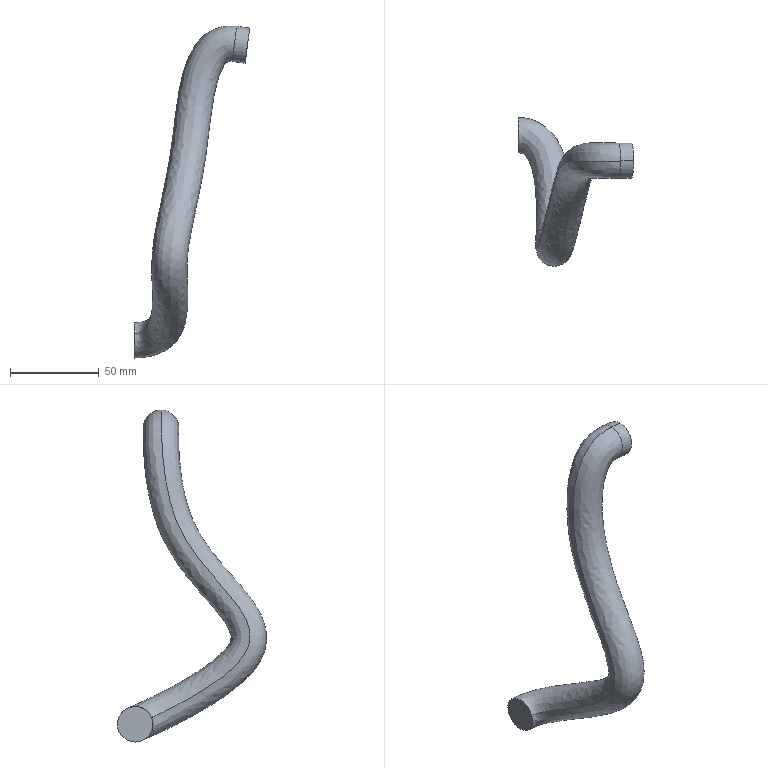Part | SolidWorks | features BaseBody 1 | 1 solid | 6 faces | box 65.187 x 84.209 x 187.357 mm | volume 76997 mm3 | cylinder 2 | plane 2 | spline 2 | commonest cylinder face diameters 20 x2